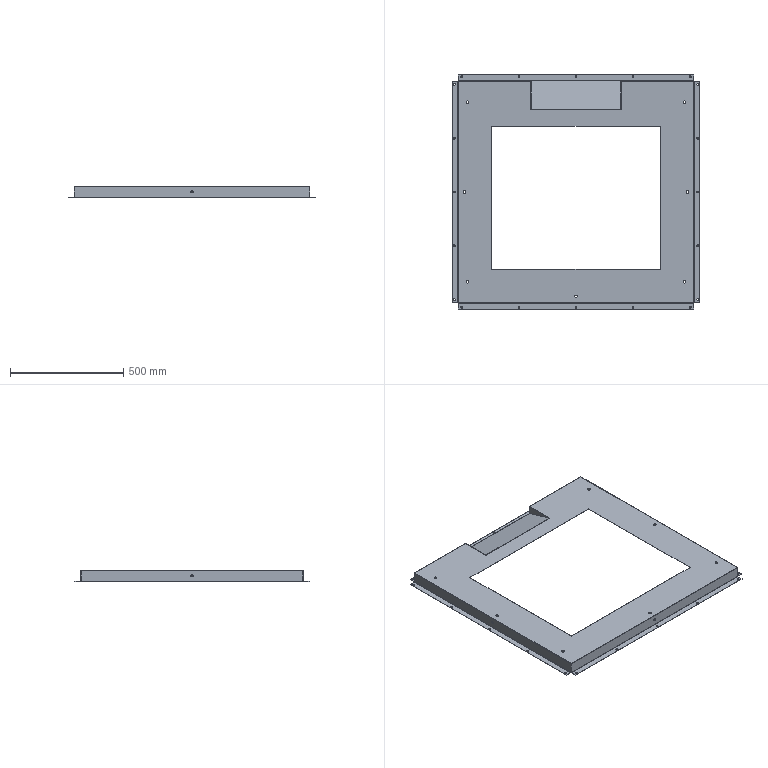Part | SolidWorks | 2 solids | 214 faces | box 1095 x 1035 x 50.189 mm | volume 845352 mm3 | plane 110 | cylinder 92 | spline 12 | commonest cylinder face diameters 7 x50 11 x14 0.4 x11 2.4 x11 10 x6